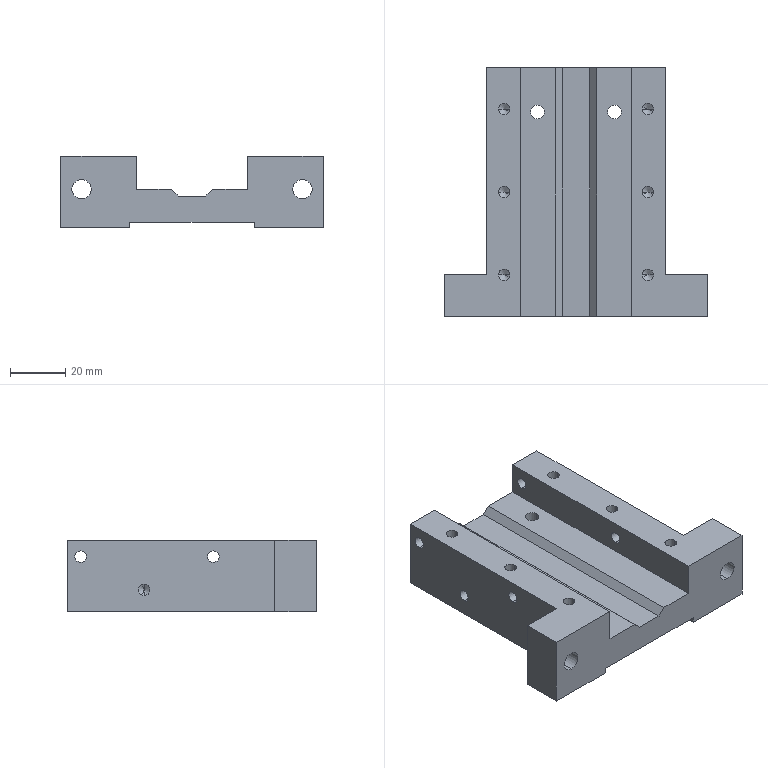Part | STEP file | magnetic tile top shaft slide seat | 1 solid | 70 faces | box 95 x 90 x 26 mm | volume 105605 mm3 | cylinder 32 | plane 22 | cone 16 | commonest cylinder face diameters 4.2 x24 5 x4 7 x4